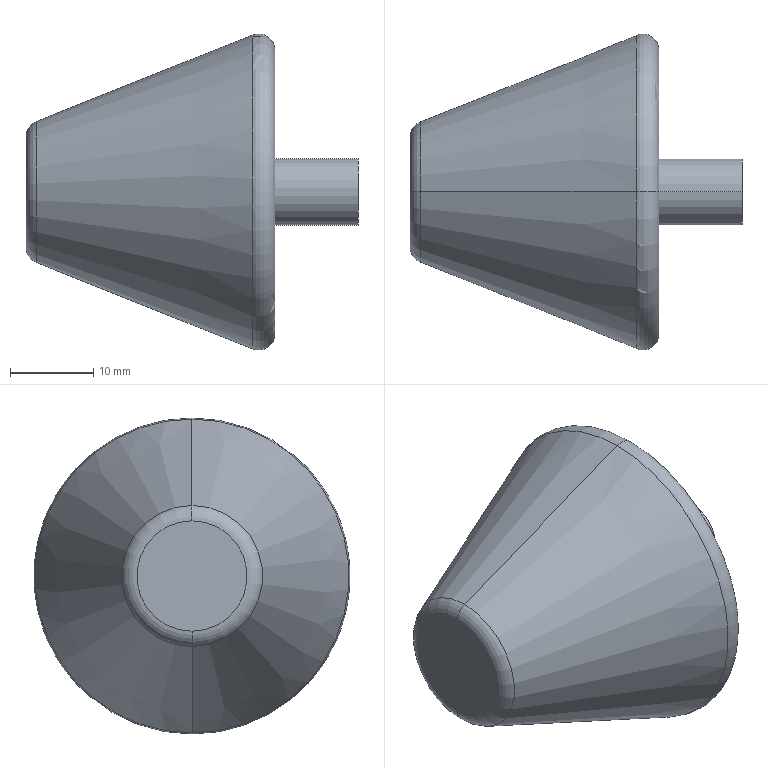Part | SolidWorks | features Fillet 2, ICE 1, Revolution 1 | 1 solid | 11 faces | box 40 x 38.092 x 38.092 mm | volume 19850 mm3 | torus 4 | plane 3 | cylinder 2 | cone 2 | commonest cylinder face diameters 8 x2
STEP:
#1=CARTESIAN_POINT('',(30.,0.,-17.046));
#2=VERTEX_POINT('',#1);
#3=CARTESIAN_POINT('',(30.,0.,17.046));
#4=VERTEX_POINT('',#3);
#5=CARTESIAN_POINT('',(30.,0.,0.));
#6=DIRECTION('',(1.,0.,0.));
#7=DIRECTION('',(0.,0.,1.));
#8=AXIS2_PLACEMENT_3D('',#5,#6,#7);
#9=CIRCLE('',#8,17.046);
#10=EDGE_CURVE('',#2,#4,#9,.T.);
#11=ORIENTED_EDGE('',*,*,#10,.F.);
#12=CARTESIAN_POINT('',(27.257,0.,-18.903));
#13=VERTEX_POINT('',#12);
#14=CARTESIAN_POINT('',(28.,0.,-17.046));
#15=DIRECTION('',(0.,1.,0.));
#16=DIRECTION('',(0.,0.,1.));
#17=AXIS2_PLACEMENT_3D('',#14,#15,#16);
#18=CIRCLE('',#17,2.);
#19=EDGE_CURVE('',#2,#13,#18,.T.);
#20=ORIENTED_EDGE('',*,*,#19,.T.);
#21=CARTESIAN_POINT('',(27.257,0.,18.903));
#22=VERTEX_POINT('',#21);
#23=CARTESIAN_POINT('',(27.257,0.,0.));
#24=DIRECTION('',(-1.,0.,0.));
#25=DIRECTION('',(0.,0.,1.));
#26=AXIS2_PLACEMENT_3D('',#23,#24,#25);
#27=CIRCLE('',#26,18.903);
#28=EDGE_CURVE('',#22,#13,#27,.T.);
#29=ORIENTED_EDGE('',*,*,#28,.F.);
#30=CARTESIAN_POINT('',(28.,0.,17.046));
#31=DIRECTION('',(0.,-1.,0.));
#32=DIRECTION('',(0.,0.,-1.));
#33=AXIS2_PLACEMENT_3D('',#30,#31,#32);
#34=CIRCLE('',#33,2.);
#35=EDGE_CURVE('',#4,#22,#34,.T.);
#36=ORIENTED_EDGE('',*,*,#35,.F.);
#37=EDGE_LOOP('',(#11,#20,#29,#36));
#38=FACE_OUTER_BOUND('',#37,.T.);
#39=CARTESIAN_POINT('',(28.,0.,0.));
#40=DIRECTION('',(-1.,0.,0.));
#41=DIRECTION('',(0.,0.,1.));
#42=AXIS2_PLACEMENT_3D('',#39,#40,#41);
#43=TOROIDAL_SURFACE('',#42,17.046,2.);
#44=ADVANCED_FACE('',(#38),#43,.T.);
#45=CARTESIAN_POINT('',(40.,0.,-4.));
#46=VERTEX_POINT('',#45);
#47=CARTESIAN_POINT('',(40.,0.,4.));
#48=VERTEX_POINT('',#47);
#49=CARTESIAN_POINT('',(40.,0.,0.));
#50=DIRECTION('',(1.,0.,0.));
#51=DIRECTION('',(0.,0.,-1.));
#52=AXIS2_PLACEMENT_3D('',#49,#50,#51);
#53=CIRCLE('',#52,4.);
#54=EDGE_CURVE('',#46,#48,#53,.T.);
#55=ORIENTED_EDGE('',*,*,#54,.F.);
#56=CARTESIAN_POINT('',(30.,0.,-4.));
#57=VERTEX_POINT('',#56);
#58=CARTESIAN_POINT('',(40.,0.,-4.));
#59=DIRECTION('',(-1.,0.,0.));
#60=VECTOR('',#59,1000.);
#61=LINE('',#58,#60);
#62=EDGE_CURVE('',#46,#57,#61,.T.);
#63=ORIENTED_EDGE('',*,*,#62,.T.);
#64=CARTESIAN_POINT('',(30.,0.,4.));
#65=VERTEX_POINT('',#64);
#66=CARTESIAN_POINT('',(30.,0.,0.));
#67=DIRECTION('',(1.,0.,0.));
#68=DIRECTION('',(0.,0.,1.));
#69=AXIS2_PLACEMENT_3D('',#66,#67,#68);
#70=CIRCLE('',#69,4.);
#71=EDGE_CURVE('',#57,#65,#70,.T.);
#72=ORIENTED_EDGE('',*,*,#71,.T.);
#73=CARTESIAN_POINT('',(40.,0.,4.));
#74=DIRECTION('',(-1.,0.,0.));
#75=VECTOR('',#74,1000.);
#76=LINE('',#73,#75);
#77=EDGE_CURVE('',#48,#65,#76,.T.);
#78=ORIENTED_EDGE('',*,*,#77,.F.);
#79=EDGE_LOOP('',(#55,#63,#72,#78));
#80=FACE_OUTER_BOUND('',#79,.T.);
#81=CARTESIAN_POINT('',(40.,0.,0.));
#82=DIRECTION('',(-1.,0.,0.));
#83=DIRECTION('',(0.,0.,1.));
#84=AXIS2_PLACEMENT_3D('',#81,#82,#83);
#85=CYLINDRICAL_SURFACE('',#84,4.);
#86=ADVANCED_FACE('',(#80),#85,.T.);
#87=CARTESIAN_POINT('',(0.,0.,6.646));
#88=VERTEX_POINT('',#87);
#89=CARTESIAN_POINT('',(0.,0.,-6.646));
#90=VERTEX_POINT('',#89);
#91=CARTESIAN_POINT('',(0.,0.,0.));
#92=DIRECTION('',(-1.,0.,0.));
#93=DIRECTION('',(0.,0.,-1.));
#94=AXIS2_PLACEMENT_3D('',#91,#92,#93);
#95=CIRCLE('',#94,6.646);
#96=EDGE_CURVE('',#88,#90,#95,.T.);
#97=ORIENTED_EDGE('',*,*,#96,.F.);
#98=CARTESIAN_POINT('',(1.257,0.,8.503));
#99=VERTEX_POINT('',#98);
#100=CARTESIAN_POINT('',(2.,0.,6.646));
#101=DIRECTION('',(0.,1.,0.));
#102=DIRECTION('',(0.,0.,1.));
#103=AXIS2_PLACEMENT_3D('',#100,#101,#102);
#104=CIRCLE('',#103,2.);
#105=EDGE_CURVE('',#88,#99,#104,.T.);
#106=ORIENTED_EDGE('',*,*,#105,.T.);
#107=CARTESIAN_POINT('',(1.257,0.,-8.503));
#108=VERTEX_POINT('',#107);
#109=CARTESIAN_POINT('',(1.257,0.,0.));
#110=DIRECTION('',(1.,0.,0.));
#111=DIRECTION('',(0.,0.,1.));
#112=AXIS2_PLACEMENT_3D('',#109,#110,#111);
#113=CIRCLE('',#112,8.503);
#114=EDGE_CURVE('',#108,#99,#113,.T.);
#115=ORIENTED_EDGE('',*,*,#114,.F.);
#116=CARTESIAN_POINT('',(2.,0.,-6.646));
#117=DIRECTION('',(0.,-1.,0.));
#118=DIRECTION('',(0.,0.,-1.));
#119=AXIS2_PLACEMENT_3D('',#116,#117,#118);
#120=CIRCLE('',#119,2.);
#121=EDGE_CURVE('',#90,#108,#120,.T.);
#122=ORIENTED_EDGE('',*,*,#121,.F.);
#123=EDGE_LOOP('',(#97,#106,#115,#122));
#124=FACE_OUTER_BOUND('',#123,.T.);
#125=CARTESIAN_POINT('',(2.,0.,0.));
#126=DIRECTION('',(1.,0.,0.));
#127=DIRECTION('',(0.,0.,-1.));
#128=AXIS2_PLACEMENT_3D('',#125,#126,#127);
#129=TOROIDAL_SURFACE('',#128,6.646,2.);
#130=ADVANCED_FACE('',(#124),#129,.T.);
#131=ORIENTED_EDGE('',*,*,#114,.T.);
#132=CARTESIAN_POINT('',(30.,0.,20.));
#133=DIRECTION('',(0.9285,0.,0.3714));
#134=VECTOR('',#133,1000.);
#135=LINE('',#132,#134);
#136=EDGE_CURVE('',#99,#22,#135,.T.);
#137=ORIENTED_EDGE('',*,*,#136,.T.);
#138=ORIENTED_EDGE('',*,*,#28,.T.);
#139=CARTESIAN_POINT('',(30.,0.,-20.));
#140=DIRECTION('',(0.9285,0.,-0.3714));
#141=VECTOR('',#140,1000.);
#142=LINE('',#139,#141);
#143=EDGE_CURVE('',#108,#13,#142,.T.);
#144=ORIENTED_EDGE('',*,*,#143,.F.);
#145=EDGE_LOOP('',(#131,#137,#138,#144));
#146=FACE_OUTER_BOUND('',#145,.T.);
#147=CARTESIAN_POINT('',(30.,0.,0.));
#148=DIRECTION('',(1.,0.,0.));
#149=DIRECTION('',(0.,0.,-1.));
#150=AXIS2_PLACEMENT_3D('',#147,#148,#149);
#151=CONICAL_SURFACE('',#150,20.,0.3805);
#152=ADVANCED_FACE('',(#146),#151,.T.);
#153=CARTESIAN_POINT('',(30.,0.,0.));
#154=DIRECTION('',(1.,0.,0.));
#155=DIRECTION('',(0.,0.,1.));
#156=AXIS2_PLACEMENT_3D('',#153,#154,#155);
#157=CIRCLE('',#156,17.046);
#158=EDGE_CURVE('',#4,#2,#157,.T.);
#159=ORIENTED_EDGE('',*,*,#158,.T.);
#160=ORIENTED_EDGE('',*,*,#10,.T.);
#161=EDGE_LOOP('',(#159,#160));
#162=FACE_OUTER_BOUND('',#161,.T.);
#163=CARTESIAN_POINT('',(30.,0.,0.));
#164=DIRECTION('',(1.,0.,0.));
#165=DIRECTION('',(0.,0.,1.));
#166=AXIS2_PLACEMENT_3D('',#163,#164,#165);
#167=CIRCLE('',#166,4.);
#168=EDGE_CURVE('',#65,#57,#167,.T.);
#169=ORIENTED_EDGE('',*,*,#168,.F.);
#170=ORIENTED_EDGE('',*,*,#71,.F.);
#171=EDGE_LOOP('',(#169,#170));
#172=FACE_BOUND('',#171,.T.);
#173=CARTESIAN_POINT('',(30.,20.,0.));
#174=DIRECTION('',(-1.,0.,0.));
#175=DIRECTION('',(0.,0.,1.));
#176=AXIS2_PLACEMENT_3D('',#173,#174,#175);
#177=PLANE('',#176);
#178=ADVANCED_FACE('',(#162,#172),#177,.F.);
#179=ORIENTED_EDGE('',*,*,#136,.F.);
#180=CARTESIAN_POINT('',(1.257,0.,0.));
#181=DIRECTION('',(1.,0.,0.));
#182=DIRECTION('',(0.,0.,1.));
#183=AXIS2_PLACEMENT_3D('',#180,#181,#182);
#184=CIRCLE('',#183,8.503);
#185=EDGE_CURVE('',#99,#108,#184,.T.);
#186=ORIENTED_EDGE('',*,*,#185,.T.);
#187=ORIENTED_EDGE('',*,*,#143,.T.);
#188=CARTESIAN_POINT('',(27.257,0.,0.));
#189=DIRECTION('',(-1.,0.,0.));
#190=DIRECTION('',(0.,0.,1.));
#191=AXIS2_PLACEMENT_3D('',#188,#189,#190);
#192=CIRCLE('',#191,18.903);
#193=EDGE_CURVE('',#13,#22,#192,.T.);
#194=ORIENTED_EDGE('',*,*,#193,.T.);
#195=EDGE_LOOP('',(#179,#186,#187,#194));
#196=FACE_OUTER_BOUND('',#195,.T.);
#197=CARTESIAN_POINT('',(30.,0.,0.));
#198=DIRECTION('',(1.,0.,0.));
#199=DIRECTION('',(0.,0.,-1.));
#200=AXIS2_PLACEMENT_3D('',#197,#198,#199);
#201=CONICAL_SURFACE('',#200,20.,0.3805);
#202=ADVANCED_FACE('',(#196),#201,.T.);
#203=CARTESIAN_POINT('',(0.,0.,0.));
#204=DIRECTION('',(-1.,0.,0.));
#205=DIRECTION('',(0.,0.,-1.));
#206=AXIS2_PLACEMENT_3D('',#203,#204,#205);
#207=CIRCLE('',#206,6.646);
#208=EDGE_CURVE('',#90,#88,#207,.T.);
#209=ORIENTED_EDGE('',*,*,#208,.T.);
#210=ORIENTED_EDGE('',*,*,#96,.T.);
#211=EDGE_LOOP('',(#209,#210));
#212=FACE_OUTER_BOUND('',#211,.T.);
#213=CARTESIAN_POINT('',(0.,0.,0.));
#214=DIRECTION('',(1.,0.,0.));
#215=DIRECTION('',(0.,0.,-1.));
#216=AXIS2_PLACEMENT_3D('',#213,#214,#215);
#217=PLANE('',#216);
#218=ADVANCED_FACE('',(#212),#217,.F.);
#219=ORIENTED_EDGE('',*,*,#105,.F.);
#220=ORIENTED_EDGE('',*,*,#208,.F.);
#221=ORIENTED_EDGE('',*,*,#121,.T.);
#222=ORIENTED_EDGE('',*,*,#185,.F.);
#223=EDGE_LOOP('',(#219,#220,#221,#222));
#224=FACE_OUTER_BOUND('',#223,.T.);
#225=CARTESIAN_POINT('',(2.,0.,0.));
#226=DIRECTION('',(1.,0.,0.));
#227=DIRECTION('',(0.,0.,-1.));
#228=AXIS2_PLACEMENT_3D('',#225,#226,#227);
#229=TOROIDAL_SURFACE('',#228,6.646,2.);
#230=ADVANCED_FACE('',(#224),#229,.T.);
#231=ORIENTED_EDGE('',*,*,#62,.F.);
#232=CARTESIAN_POINT('',(40.,0.,0.));
#233=DIRECTION('',(1.,0.,0.));
#234=DIRECTION('',(0.,0.,-1.));
#235=AXIS2_PLACEMENT_3D('',#232,#233,#234);
#236=CIRCLE('',#235,4.);
#237=EDGE_CURVE('',#48,#46,#236,.T.);
#238=ORIENTED_EDGE('',*,*,#237,.F.);
#239=ORIENTED_EDGE('',*,*,#77,.T.);
#240=ORIENTED_EDGE('',*,*,#168,.T.);
#241=EDGE_LOOP('',(#231,#238,#239,#240));
#242=FACE_OUTER_BOUND('',#241,.T.);
#243=CARTESIAN_POINT('',(40.,0.,0.));
#244=DIRECTION('',(-1.,0.,0.));
#245=DIRECTION('',(0.,0.,1.));
#246=AXIS2_PLACEMENT_3D('',#243,#244,#245);
#247=CYLINDRICAL_SURFACE('',#246,4.);
#248=ADVANCED_FACE('',(#242),#247,.T.);
#249=ORIENTED_EDGE('',*,*,#237,.T.);
#250=ORIENTED_EDGE('',*,*,#54,.T.);
#251=EDGE_LOOP('',(#249,#250));
#252=FACE_OUTER_BOUND('',#251,.T.);
#253=CARTESIAN_POINT('',(40.,0.,0.));
#254=DIRECTION('',(1.,0.,0.));
#255=DIRECTION('',(0.,0.,-1.));
#256=AXIS2_PLACEMENT_3D('',#253,#254,#255);
#257=PLANE('',#256);
#258=ADVANCED_FACE('',(#252),#257,.T.);
#259=ORIENTED_EDGE('',*,*,#19,.F.);
#260=ORIENTED_EDGE('',*,*,#158,.F.);
#261=ORIENTED_EDGE('',*,*,#35,.T.);
#262=ORIENTED_EDGE('',*,*,#193,.F.);
#263=EDGE_LOOP('',(#259,#260,#261,#262));
#264=FACE_OUTER_BOUND('',#263,.T.);
#265=CARTESIAN_POINT('',(28.,0.,0.));
#266=DIRECTION('',(-1.,0.,0.));
#267=DIRECTION('',(0.,0.,1.));
#268=AXIS2_PLACEMENT_3D('',#265,#266,#267);
#269=TOROIDAL_SURFACE('',#268,17.046,2.);
#270=ADVANCED_FACE('',(#264),#269,.T.);
#271=CLOSED_SHELL('',(#44,#86,#130,#152,#178,#202,#218,#230,#248,#258,#270));
#272=MANIFOLD_SOLID_BREP('',#271);
#273=CARTESIAN_POINT('',(0.,0.,0.));
#274=DIRECTION('',(0.,0.,1.));
#275=DIRECTION('',(1.,0.,0.));
#276=AXIS2_PLACEMENT_3D('',#273,#274,#275);
#277=(LENGTH_UNIT()NAMED_UNIT(*)SI_UNIT(.MILLI.,.METRE.));
#278=UNCERTAINTY_MEASURE_WITH_UNIT(LENGTH_MEASURE(0.00001),#277,'','');
#279=(NAMED_UNIT(*)PLANE_ANGLE_UNIT()SI_UNIT($,.RADIAN.));
#280=(NAMED_UNIT(*)SI_UNIT($,.STERADIAN.)SOLID_ANGLE_UNIT());
#281=(GEOMETRIC_REPRESENTATION_CONTEXT(3)GLOBAL_UNCERTAINTY_ASSIGNED_CONTEXT((#278))GLOBAL_UNIT_ASSIGNED_CONTEXT((#277,#279,#280))REPRESENTATION_CONTEXT('',''));
#282=ADVANCED_BREP_SHAPE_REPRESENTATION('',(#272,#276),#281);